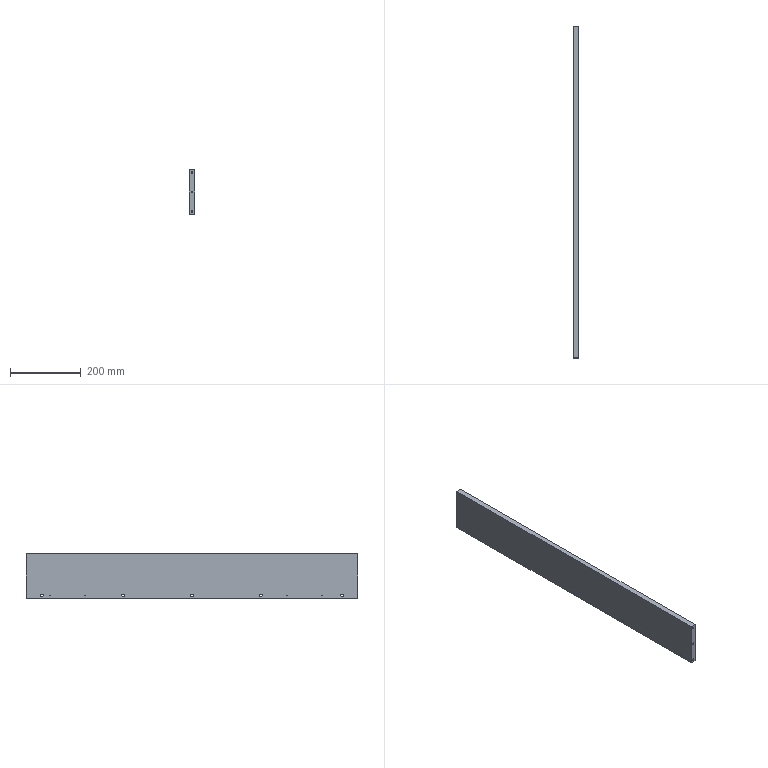Part | STEP file | 0244_209_Plate | 1 solid | 63 faces | box 15 x 940 x 125 mm | volume 1754241 mm3 | cylinder 40 | cone 12 | plane 11 | commonest cylinder face diameters 5 x12 7 x10 11 x10 2.5 x8